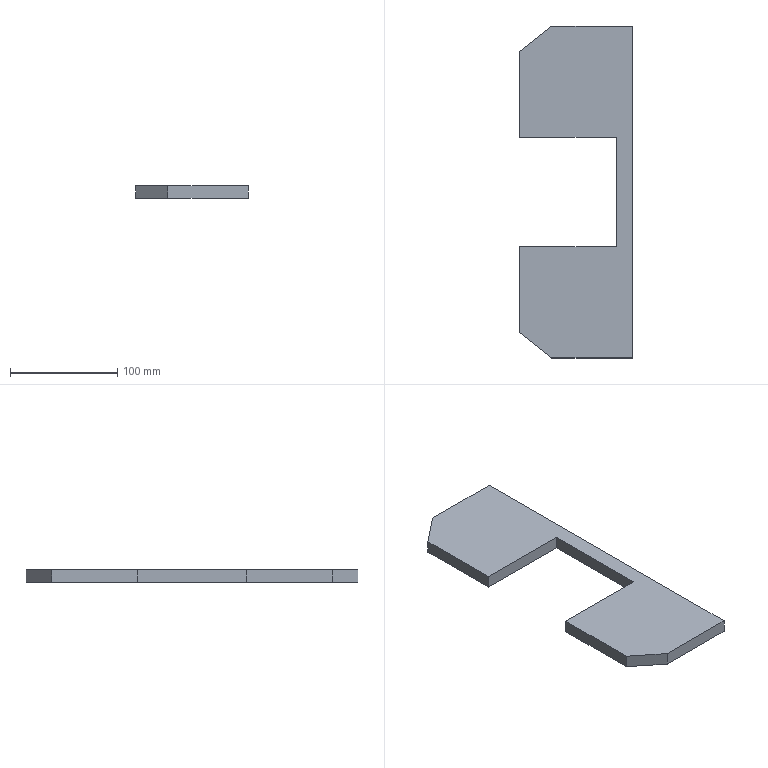Part | SolidWorks | features Extrusion 1, ICE 1 | 1 solid | 12 faces | box 105 x 310 x 12 mm | volume 271800 mm3 | plane 12
STEP:
#1=CARTESIAN_POINT('',(-7.5,-51.,6.));
#2=VERTEX_POINT('',#1);
#3=CARTESIAN_POINT('',(-7.5,-51.,-6.));
#4=VERTEX_POINT('',#3);
#5=CARTESIAN_POINT('',(-7.5,-51.,6.));
#6=DIRECTION('',(0.,0.,-1.));
#7=VECTOR('',#6,1000.);
#8=LINE('',#5,#7);
#9=EDGE_CURVE('',#2,#4,#8,.T.);
#10=ORIENTED_EDGE('',*,*,#9,.F.);
#11=CARTESIAN_POINT('',(-7.5,51.,6.));
#12=VERTEX_POINT('',#11);
#13=CARTESIAN_POINT('',(-7.5,155.,6.));
#14=DIRECTION('',(0.,-1.,0.));
#15=VECTOR('',#14,1000.);
#16=LINE('',#13,#15);
#17=EDGE_CURVE('',#12,#2,#16,.T.);
#18=ORIENTED_EDGE('',*,*,#17,.F.);
#19=CARTESIAN_POINT('',(-7.5,51.,-6.));
#20=VERTEX_POINT('',#19);
#21=CARTESIAN_POINT('',(-7.5,51.,6.));
#22=DIRECTION('',(0.,0.,-1.));
#23=VECTOR('',#22,1000.);
#24=LINE('',#21,#23);
#25=EDGE_CURVE('',#12,#20,#24,.T.);
#26=ORIENTED_EDGE('',*,*,#25,.T.);
#27=CARTESIAN_POINT('',(-7.5,155.,-6.));
#28=DIRECTION('',(0.,-1.,0.));
#29=VECTOR('',#28,1000.);
#30=LINE('',#27,#29);
#31=EDGE_CURVE('',#20,#4,#30,.T.);
#32=ORIENTED_EDGE('',*,*,#31,.T.);
#33=EDGE_LOOP('',(#10,#18,#26,#32));
#34=FACE_OUTER_BOUND('',#33,.T.);
#35=CARTESIAN_POINT('',(-7.5,155.,6.));
#36=DIRECTION('',(1.,0.,0.));
#37=DIRECTION('',(0.,0.,-1.));
#38=AXIS2_PLACEMENT_3D('',#35,#36,#37);
#39=PLANE('',#38);
#40=ADVANCED_FACE('',(#34),#39,.F.);
#41=CARTESIAN_POINT('',(7.5,155.,-6.));
#42=VERTEX_POINT('',#41);
#43=CARTESIAN_POINT('',(-67.5,155.,-6.));
#44=VERTEX_POINT('',#43);
#45=CARTESIAN_POINT('',(7.5,155.,-6.));
#46=DIRECTION('',(-1.,0.,0.));
#47=VECTOR('',#46,1000.);
#48=LINE('',#45,#47);
#49=EDGE_CURVE('',#42,#44,#48,.T.);
#50=ORIENTED_EDGE('',*,*,#49,.T.);
#51=CARTESIAN_POINT('',(-67.5,155.,6.));
#52=VERTEX_POINT('',#51);
#53=CARTESIAN_POINT('',(-67.5,155.,6.));
#54=DIRECTION('',(0.,0.,-1.));
#55=VECTOR('',#54,1000.);
#56=LINE('',#53,#55);
#57=EDGE_CURVE('',#52,#44,#56,.T.);
#58=ORIENTED_EDGE('',*,*,#57,.F.);
#59=CARTESIAN_POINT('',(7.5,155.,6.));
#60=VERTEX_POINT('',#59);
#61=CARTESIAN_POINT('',(7.5,155.,6.));
#62=DIRECTION('',(-1.,0.,0.));
#63=VECTOR('',#62,1000.);
#64=LINE('',#61,#63);
#65=EDGE_CURVE('',#60,#52,#64,.T.);
#66=ORIENTED_EDGE('',*,*,#65,.F.);
#67=CARTESIAN_POINT('',(7.5,155.,6.));
#68=DIRECTION('',(0.,0.,-1.));
#69=VECTOR('',#68,1000.);
#70=LINE('',#67,#69);
#71=EDGE_CURVE('',#60,#42,#70,.T.);
#72=ORIENTED_EDGE('',*,*,#71,.T.);
#73=EDGE_LOOP('',(#50,#58,#66,#72));
#74=FACE_OUTER_BOUND('',#73,.T.);
#75=CARTESIAN_POINT('',(7.5,155.,6.));
#76=DIRECTION('',(0.,-1.,0.));
#77=DIRECTION('',(0.,0.,-1.));
#78=AXIS2_PLACEMENT_3D('',#75,#76,#77);
#79=PLANE('',#78);
#80=ADVANCED_FACE('',(#74),#79,.F.);
#81=CARTESIAN_POINT('',(-67.5,-155.,-6.));
#82=VERTEX_POINT('',#81);
#83=CARTESIAN_POINT('',(7.5,-155.,-6.));
#84=VERTEX_POINT('',#83);
#85=CARTESIAN_POINT('',(-7.5,-155.,-6.));
#86=DIRECTION('',(1.,0.,0.));
#87=VECTOR('',#86,1000.);
#88=LINE('',#85,#87);
#89=EDGE_CURVE('',#82,#84,#88,.T.);
#90=ORIENTED_EDGE('',*,*,#89,.T.);
#91=CARTESIAN_POINT('',(7.5,-155.,6.));
#92=VERTEX_POINT('',#91);
#93=CARTESIAN_POINT('',(7.5,-155.,6.));
#94=DIRECTION('',(0.,0.,-1.));
#95=VECTOR('',#94,1000.);
#96=LINE('',#93,#95);
#97=EDGE_CURVE('',#92,#84,#96,.T.);
#98=ORIENTED_EDGE('',*,*,#97,.F.);
#99=CARTESIAN_POINT('',(-67.5,-155.,6.));
#100=VERTEX_POINT('',#99);
#101=CARTESIAN_POINT('',(-7.5,-155.,6.));
#102=DIRECTION('',(1.,0.,0.));
#103=VECTOR('',#102,1000.);
#104=LINE('',#101,#103);
#105=EDGE_CURVE('',#100,#92,#104,.T.);
#106=ORIENTED_EDGE('',*,*,#105,.F.);
#107=CARTESIAN_POINT('',(-67.5,-155.,6.));
#108=DIRECTION('',(0.,0.,-1.));
#109=VECTOR('',#108,1000.);
#110=LINE('',#107,#109);
#111=EDGE_CURVE('',#100,#82,#110,.T.);
#112=ORIENTED_EDGE('',*,*,#111,.T.);
#113=EDGE_LOOP('',(#90,#98,#106,#112));
#114=FACE_OUTER_BOUND('',#113,.T.);
#115=CARTESIAN_POINT('',(-7.5,-155.,6.));
#116=DIRECTION('',(0.,1.,0.));
#117=DIRECTION('',(0.,0.,1.));
#118=AXIS2_PLACEMENT_3D('',#115,#116,#117);
#119=PLANE('',#118);
#120=ADVANCED_FACE('',(#114),#119,.F.);
#121=CARTESIAN_POINT('',(7.5,-155.,-6.));
#122=DIRECTION('',(0.,1.,0.));
#123=VECTOR('',#122,1000.);
#124=LINE('',#121,#123);
#125=EDGE_CURVE('',#84,#42,#124,.T.);
#126=ORIENTED_EDGE('',*,*,#125,.T.);
#127=ORIENTED_EDGE('',*,*,#71,.F.);
#128=CARTESIAN_POINT('',(7.5,-155.,6.));
#129=DIRECTION('',(0.,1.,0.));
#130=VECTOR('',#129,1000.);
#131=LINE('',#128,#130);
#132=EDGE_CURVE('',#92,#60,#131,.T.);
#133=ORIENTED_EDGE('',*,*,#132,.F.);
#134=ORIENTED_EDGE('',*,*,#97,.T.);
#135=EDGE_LOOP('',(#126,#127,#133,#134));
#136=FACE_OUTER_BOUND('',#135,.T.);
#137=CARTESIAN_POINT('',(7.5,-155.,6.));
#138=DIRECTION('',(-1.,0.,0.));
#139=DIRECTION('',(0.,0.,1.));
#140=AXIS2_PLACEMENT_3D('',#137,#138,#139);
#141=PLANE('',#140);
#142=ADVANCED_FACE('',(#136),#141,.F.);
#143=ORIENTED_EDGE('',*,*,#65,.T.);
#144=CARTESIAN_POINT('',(-97.5,131.,6.));
#145=VERTEX_POINT('',#144);
#146=CARTESIAN_POINT('',(-67.5,155.,6.));
#147=DIRECTION('',(-0.7809,-0.6247,0.));
#148=VECTOR('',#147,1000.);
#149=LINE('',#146,#148);
#150=EDGE_CURVE('',#52,#145,#149,.T.);
#151=ORIENTED_EDGE('',*,*,#150,.T.);
#152=CARTESIAN_POINT('',(-97.5,51.,6.));
#153=VERTEX_POINT('',#152);
#154=CARTESIAN_POINT('',(-97.5,131.,6.));
#155=DIRECTION('',(0.,-1.,0.));
#156=VECTOR('',#155,1000.);
#157=LINE('',#154,#156);
#158=EDGE_CURVE('',#145,#153,#157,.T.);
#159=ORIENTED_EDGE('',*,*,#158,.T.);
#160=CARTESIAN_POINT('',(-97.5,51.,6.));
#161=DIRECTION('',(1.,0.,0.));
#162=VECTOR('',#161,1000.);
#163=LINE('',#160,#162);
#164=EDGE_CURVE('',#153,#12,#163,.T.);
#165=ORIENTED_EDGE('',*,*,#164,.T.);
#166=ORIENTED_EDGE('',*,*,#17,.T.);
#167=CARTESIAN_POINT('',(-97.5,-51.,6.));
#168=VERTEX_POINT('',#167);
#169=CARTESIAN_POINT('',(-97.5,-51.,6.));
#170=DIRECTION('',(-1.,0.,0.));
#171=VECTOR('',#170,1000.);
#172=LINE('',#169,#171);
#173=EDGE_CURVE('',#2,#168,#172,.T.);
#174=ORIENTED_EDGE('',*,*,#173,.T.);
#175=CARTESIAN_POINT('',(-97.5,-131.,6.));
#176=VERTEX_POINT('',#175);
#177=CARTESIAN_POINT('',(-97.5,-131.,6.));
#178=DIRECTION('',(0.,-1.,0.));
#179=VECTOR('',#178,1000.);
#180=LINE('',#177,#179);
#181=EDGE_CURVE('',#168,#176,#180,.T.);
#182=ORIENTED_EDGE('',*,*,#181,.T.);
#183=CARTESIAN_POINT('',(-67.5,-155.,6.));
#184=DIRECTION('',(0.7809,-0.6247,0.));
#185=VECTOR('',#184,1000.);
#186=LINE('',#183,#185);
#187=EDGE_CURVE('',#176,#100,#186,.T.);
#188=ORIENTED_EDGE('',*,*,#187,.T.);
#189=ORIENTED_EDGE('',*,*,#105,.T.);
#190=ORIENTED_EDGE('',*,*,#132,.T.);
#191=EDGE_LOOP('',(#143,#151,#159,#165,#166,#174,#182,#188,#189,#190));
#192=FACE_OUTER_BOUND('',#191,.T.);
#193=CARTESIAN_POINT('',(-7.5,155.,6.));
#194=DIRECTION('',(0.,0.,1.));
#195=DIRECTION('',(1.,0.,0.));
#196=AXIS2_PLACEMENT_3D('',#193,#194,#195);
#197=PLANE('',#196);
#198=ADVANCED_FACE('',(#192),#197,.T.);
#199=ORIENTED_EDGE('',*,*,#49,.F.);
#200=ORIENTED_EDGE('',*,*,#125,.F.);
#201=ORIENTED_EDGE('',*,*,#89,.F.);
#202=CARTESIAN_POINT('',(-97.5,-131.,-6.));
#203=VERTEX_POINT('',#202);
#204=CARTESIAN_POINT('',(-67.5,-155.,-6.));
#205=DIRECTION('',(0.7809,-0.6247,0.));
#206=VECTOR('',#205,1000.);
#207=LINE('',#204,#206);
#208=EDGE_CURVE('',#203,#82,#207,.T.);
#209=ORIENTED_EDGE('',*,*,#208,.F.);
#210=CARTESIAN_POINT('',(-97.5,-51.,-6.));
#211=VERTEX_POINT('',#210);
#212=CARTESIAN_POINT('',(-97.5,-131.,-6.));
#213=DIRECTION('',(0.,-1.,0.));
#214=VECTOR('',#213,1000.);
#215=LINE('',#212,#214);
#216=EDGE_CURVE('',#211,#203,#215,.T.);
#217=ORIENTED_EDGE('',*,*,#216,.F.);
#218=CARTESIAN_POINT('',(-97.5,-51.,-6.));
#219=DIRECTION('',(-1.,0.,0.));
#220=VECTOR('',#219,1000.);
#221=LINE('',#218,#220);
#222=EDGE_CURVE('',#4,#211,#221,.T.);
#223=ORIENTED_EDGE('',*,*,#222,.F.);
#224=ORIENTED_EDGE('',*,*,#31,.F.);
#225=CARTESIAN_POINT('',(-97.5,51.,-6.));
#226=VERTEX_POINT('',#225);
#227=CARTESIAN_POINT('',(-97.5,51.,-6.));
#228=DIRECTION('',(1.,0.,0.));
#229=VECTOR('',#228,1000.);
#230=LINE('',#227,#229);
#231=EDGE_CURVE('',#226,#20,#230,.T.);
#232=ORIENTED_EDGE('',*,*,#231,.F.);
#233=CARTESIAN_POINT('',(-97.5,131.,-6.));
#234=VERTEX_POINT('',#233);
#235=CARTESIAN_POINT('',(-97.5,131.,-6.));
#236=DIRECTION('',(0.,-1.,0.));
#237=VECTOR('',#236,1000.);
#238=LINE('',#235,#237);
#239=EDGE_CURVE('',#234,#226,#238,.T.);
#240=ORIENTED_EDGE('',*,*,#239,.F.);
#241=CARTESIAN_POINT('',(-67.5,155.,-6.));
#242=DIRECTION('',(-0.7809,-0.6247,0.));
#243=VECTOR('',#242,1000.);
#244=LINE('',#241,#243);
#245=EDGE_CURVE('',#44,#234,#244,.T.);
#246=ORIENTED_EDGE('',*,*,#245,.F.);
#247=EDGE_LOOP('',(#199,#200,#201,#209,#217,#223,#224,#232,#240,#246));
#248=FACE_OUTER_BOUND('',#247,.T.);
#249=CARTESIAN_POINT('',(-7.5,155.,-6.));
#250=DIRECTION('',(0.,0.,1.));
#251=DIRECTION('',(1.,0.,0.));
#252=AXIS2_PLACEMENT_3D('',#249,#250,#251);
#253=PLANE('',#252);
#254=ADVANCED_FACE('',(#248),#253,.F.);
#255=ORIENTED_EDGE('',*,*,#245,.T.);
#256=CARTESIAN_POINT('',(-97.5,131.,6.));
#257=DIRECTION('',(0.,0.,-1.));
#258=VECTOR('',#257,1000.);
#259=LINE('',#256,#258);
#260=EDGE_CURVE('',#145,#234,#259,.T.);
#261=ORIENTED_EDGE('',*,*,#260,.F.);
#262=ORIENTED_EDGE('',*,*,#150,.F.);
#263=ORIENTED_EDGE('',*,*,#57,.T.);
#264=EDGE_LOOP('',(#255,#261,#262,#263));
#265=FACE_OUTER_BOUND('',#264,.T.);
#266=CARTESIAN_POINT('',(-67.5,155.,6.));
#267=DIRECTION('',(0.6247,-0.7809,0.));
#268=DIRECTION('',(0.7809,0.6247,0.));
#269=AXIS2_PLACEMENT_3D('',#266,#267,#268);
#270=PLANE('',#269);
#271=ADVANCED_FACE('',(#265),#270,.F.);
#272=ORIENTED_EDGE('',*,*,#239,.T.);
#273=CARTESIAN_POINT('',(-97.5,51.,6.));
#274=DIRECTION('',(0.,0.,-1.));
#275=VECTOR('',#274,1000.);
#276=LINE('',#273,#275);
#277=EDGE_CURVE('',#153,#226,#276,.T.);
#278=ORIENTED_EDGE('',*,*,#277,.F.);
#279=ORIENTED_EDGE('',*,*,#158,.F.);
#280=ORIENTED_EDGE('',*,*,#260,.T.);
#281=EDGE_LOOP('',(#272,#278,#279,#280));
#282=FACE_OUTER_BOUND('',#281,.T.);
#283=CARTESIAN_POINT('',(-97.5,131.,6.));
#284=DIRECTION('',(1.,0.,0.));
#285=DIRECTION('',(0.,1.,0.));
#286=AXIS2_PLACEMENT_3D('',#283,#284,#285);
#287=PLANE('',#286);
#288=ADVANCED_FACE('',(#282),#287,.F.);
#289=ORIENTED_EDGE('',*,*,#231,.T.);
#290=ORIENTED_EDGE('',*,*,#25,.F.);
#291=ORIENTED_EDGE('',*,*,#164,.F.);
#292=ORIENTED_EDGE('',*,*,#277,.T.);
#293=EDGE_LOOP('',(#289,#290,#291,#292));
#294=FACE_OUTER_BOUND('',#293,.T.);
#295=CARTESIAN_POINT('',(-97.5,51.,6.));
#296=DIRECTION('',(0.,1.,0.));
#297=DIRECTION('',(-1.,0.,0.));
#298=AXIS2_PLACEMENT_3D('',#295,#296,#297);
#299=PLANE('',#298);
#300=ADVANCED_FACE('',(#294),#299,.F.);
#301=ORIENTED_EDGE('',*,*,#222,.T.);
#302=CARTESIAN_POINT('',(-97.5,-51.,6.));
#303=DIRECTION('',(0.,0.,-1.));
#304=VECTOR('',#303,1000.);
#305=LINE('',#302,#304);
#306=EDGE_CURVE('',#168,#211,#305,.T.);
#307=ORIENTED_EDGE('',*,*,#306,.F.);
#308=ORIENTED_EDGE('',*,*,#173,.F.);
#309=ORIENTED_EDGE('',*,*,#9,.T.);
#310=EDGE_LOOP('',(#301,#307,#308,#309));
#311=FACE_OUTER_BOUND('',#310,.T.);
#312=CARTESIAN_POINT('',(-97.5,-51.,6.));
#313=DIRECTION('',(0.,-1.,0.));
#314=DIRECTION('',(1.,0.,0.));
#315=AXIS2_PLACEMENT_3D('',#312,#313,#314);
#316=PLANE('',#315);
#317=ADVANCED_FACE('',(#311),#316,.F.);
#318=ORIENTED_EDGE('',*,*,#216,.T.);
#319=CARTESIAN_POINT('',(-97.5,-131.,6.));
#320=DIRECTION('',(0.,0.,-1.));
#321=VECTOR('',#320,1000.);
#322=LINE('',#319,#321);
#323=EDGE_CURVE('',#176,#203,#322,.T.);
#324=ORIENTED_EDGE('',*,*,#323,.F.);
#325=ORIENTED_EDGE('',*,*,#181,.F.);
#326=ORIENTED_EDGE('',*,*,#306,.T.);
#327=EDGE_LOOP('',(#318,#324,#325,#326));
#328=FACE_OUTER_BOUND('',#327,.T.);
#329=CARTESIAN_POINT('',(-97.5,-131.,6.));
#330=DIRECTION('',(1.,0.,0.));
#331=DIRECTION('',(0.,1.,0.));
#332=AXIS2_PLACEMENT_3D('',#329,#330,#331);
#333=PLANE('',#332);
#334=ADVANCED_FACE('',(#328),#333,.F.);
#335=ORIENTED_EDGE('',*,*,#208,.T.);
#336=ORIENTED_EDGE('',*,*,#111,.F.);
#337=ORIENTED_EDGE('',*,*,#187,.F.);
#338=ORIENTED_EDGE('',*,*,#323,.T.);
#339=EDGE_LOOP('',(#335,#336,#337,#338));
#340=FACE_OUTER_BOUND('',#339,.T.);
#341=CARTESIAN_POINT('',(-67.5,-155.,6.));
#342=DIRECTION('',(0.6247,0.7809,0.));
#343=DIRECTION('',(-0.7809,0.6247,0.));
#344=AXIS2_PLACEMENT_3D('',#341,#342,#343);
#345=PLANE('',#344);
#346=ADVANCED_FACE('',(#340),#345,.F.);
#347=CLOSED_SHELL('',(#40,#80,#120,#142,#198,#254,#271,#288,#300,#317,#334,#346));
#348=MANIFOLD_SOLID_BREP('',#347);
#349=CARTESIAN_POINT('',(0.,0.,0.));
#350=DIRECTION('',(0.,0.,1.));
#351=DIRECTION('',(1.,0.,0.));
#352=AXIS2_PLACEMENT_3D('',#349,#350,#351);
#353=(LENGTH_UNIT()NAMED_UNIT(*)SI_UNIT(.MILLI.,.METRE.));
#354=UNCERTAINTY_MEASURE_WITH_UNIT(LENGTH_MEASURE(0.00001),#353,'','');
#355=(NAMED_UNIT(*)PLANE_ANGLE_UNIT()SI_UNIT($,.RADIAN.));
#356=(NAMED_UNIT(*)SI_UNIT($,.STERADIAN.)SOLID_ANGLE_UNIT());
#357=(GEOMETRIC_REPRESENTATION_CONTEXT(3)GLOBAL_UNCERTAINTY_ASSIGNED_CONTEXT((#354))GLOBAL_UNIT_ASSIGNED_CONTEXT((#353,#355,#356))REPRESENTATION_CONTEXT('',''));
#358=ADVANCED_BREP_SHAPE_REPRESENTATION('',(#348,#352),#357);